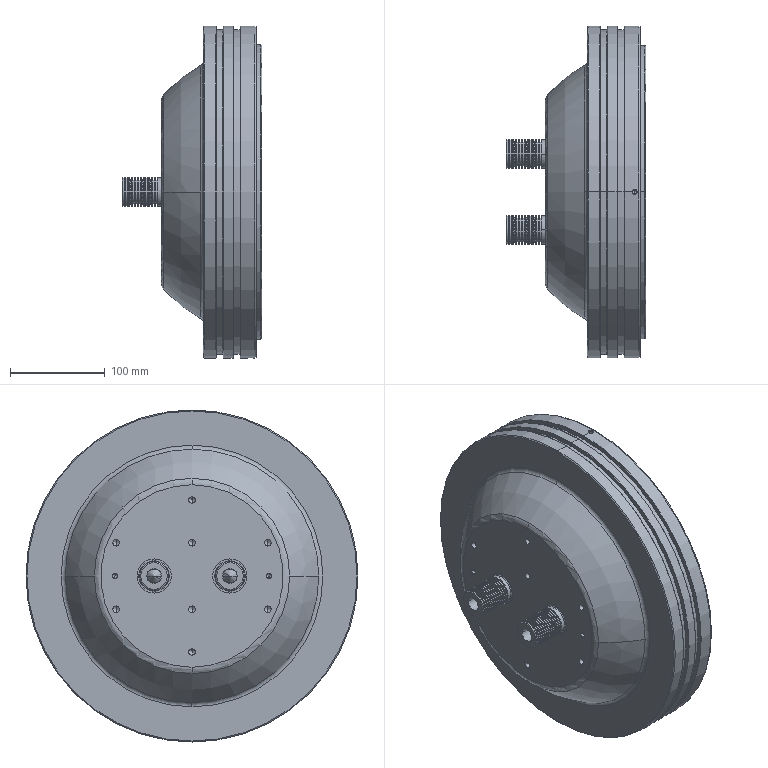Part | NX | features BREP 1 | 1 solid | 534 faces | box 147.5 x 350 x 350 mm | volume 7091284 mm3 | cylinder 174 | cone 168 | spline 79 | plane 71 | torus 40 | sphere 2 | commonest cylinder face diameters 30 x52 26 x48 6.8 x18 4.2 x16 8.5 x8 350 x6